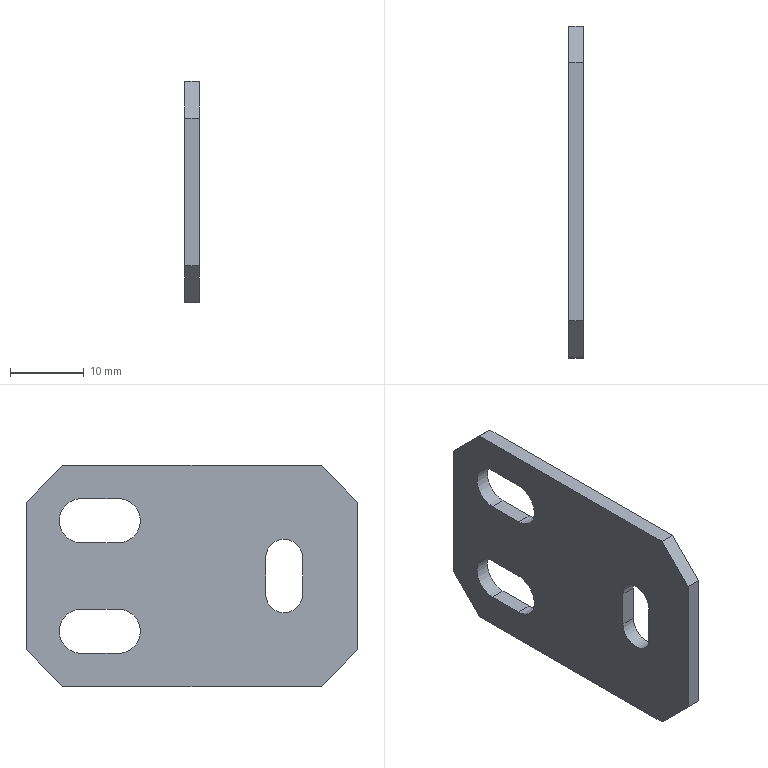Part | NX | features 5003_214_Bracket 2 | 1 solid | 22 faces | box 2 x 45 x 30 mm | volume 2278 mm3 | plane 16 | cylinder 6 | commonest cylinder face diameters 6 x4 5 x2
STEP:
#1=CARTESIAN_POINT('',(-198.775,-594.1,-44.5));
#2=VERTEX_POINT('',#1);
#3=CARTESIAN_POINT('',(-198.775,-594.1,-39.5));
#4=VERTEX_POINT('',#3);
#5=CARTESIAN_POINT('',(-198.775,-594.1,-44.5));
#6=DIRECTION('',(0.,0.,1.));
#7=VECTOR('',#6,1000.);
#8=LINE('',#5,#7);
#9=EDGE_CURVE('',#2,#4,#8,.T.);
#10=ORIENTED_EDGE('',*,*,#9,.F.);
#11=CARTESIAN_POINT('',(-198.775,-589.1,-44.5));
#12=VERTEX_POINT('',#11);
#13=CARTESIAN_POINT('',(-198.775,-591.6,-44.5));
#14=DIRECTION('',(-1.,0.,0.));
#15=DIRECTION('',(0.,0.,1.));
#16=AXIS2_PLACEMENT_3D('',#13,#14,#15);
#17=CIRCLE('',#16,2.5);
#18=EDGE_CURVE('',#12,#2,#17,.T.);
#19=ORIENTED_EDGE('',*,*,#18,.F.);
#20=CARTESIAN_POINT('',(-198.775,-589.1,-39.5));
#21=VERTEX_POINT('',#20);
#22=CARTESIAN_POINT('',(-198.775,-589.1,-44.5));
#23=DIRECTION('',(0.,0.,-1.));
#24=VECTOR('',#23,1000.);
#25=LINE('',#22,#24);
#26=EDGE_CURVE('',#21,#12,#25,.T.);
#27=ORIENTED_EDGE('',*,*,#26,.F.);
#28=CARTESIAN_POINT('',(-198.775,-591.6,-39.5));
#29=DIRECTION('',(-1.,0.,0.));
#30=DIRECTION('',(0.,0.,1.));
#31=AXIS2_PLACEMENT_3D('',#28,#29,#30);
#32=CIRCLE('',#31,2.5);
#33=EDGE_CURVE('',#4,#21,#32,.T.);
#34=ORIENTED_EDGE('',*,*,#33,.F.);
#35=EDGE_LOOP('',(#10,#19,#27,#34));
#36=FACE_BOUND('',#35,.T.);
#37=CARTESIAN_POINT('',(-198.775,-569.1,-52.5));
#38=VERTEX_POINT('',#37);
#39=CARTESIAN_POINT('',(-198.775,-569.1,-46.5));
#40=VERTEX_POINT('',#39);
#41=CARTESIAN_POINT('',(-198.775,-569.1,-49.5));
#42=DIRECTION('',(-1.,0.,0.));
#43=DIRECTION('',(0.,0.,1.));
#44=AXIS2_PLACEMENT_3D('',#41,#42,#43);
#45=CIRCLE('',#44,3.);
#46=EDGE_CURVE('',#38,#40,#45,.T.);
#47=ORIENTED_EDGE('',*,*,#46,.F.);
#48=CARTESIAN_POINT('',(-198.775,-564.1,-52.5));
#49=VERTEX_POINT('',#48);
#50=CARTESIAN_POINT('',(-198.775,-569.1,-52.5));
#51=DIRECTION('',(0.,-1.,0.));
#52=VECTOR('',#51,1000.);
#53=LINE('',#50,#52);
#54=EDGE_CURVE('',#49,#38,#53,.T.);
#55=ORIENTED_EDGE('',*,*,#54,.F.);
#56=CARTESIAN_POINT('',(-198.775,-564.1,-46.5));
#57=VERTEX_POINT('',#56);
#58=CARTESIAN_POINT('',(-198.775,-564.1,-49.5));
#59=DIRECTION('',(-1.,0.,0.));
#60=DIRECTION('',(0.,0.,1.));
#61=AXIS2_PLACEMENT_3D('',#58,#59,#60);
#62=CIRCLE('',#61,3.);
#63=EDGE_CURVE('',#57,#49,#62,.T.);
#64=ORIENTED_EDGE('',*,*,#63,.F.);
#65=CARTESIAN_POINT('',(-198.775,-564.1,-46.5));
#66=DIRECTION('',(0.,1.,0.));
#67=VECTOR('',#66,1000.);
#68=LINE('',#65,#67);
#69=EDGE_CURVE('',#40,#57,#68,.T.);
#70=ORIENTED_EDGE('',*,*,#69,.F.);
#71=EDGE_LOOP('',(#47,#55,#64,#70));
#72=FACE_BOUND('',#71,.T.);
#73=CARTESIAN_POINT('',(-198.775,-601.6,-52.));
#74=VERTEX_POINT('',#73);
#75=CARTESIAN_POINT('',(-198.775,-601.6,-32.));
#76=VERTEX_POINT('',#75);
#77=CARTESIAN_POINT('',(-198.775,-601.6,-27.));
#78=DIRECTION('',(0.,0.,1.));
#79=VECTOR('',#78,1000.);
#80=LINE('',#77,#79);
#81=EDGE_CURVE('',#74,#76,#80,.T.);
#82=ORIENTED_EDGE('',*,*,#81,.T.);
#83=CARTESIAN_POINT('',(-198.775,-596.6,-27.));
#84=VERTEX_POINT('',#83);
#85=CARTESIAN_POINT('',(-198.775,-596.6,-27.));
#86=DIRECTION('',(0.,-0.7071,-0.7071));
#87=VECTOR('',#86,1000.);
#88=LINE('',#85,#87);
#89=EDGE_CURVE('',#76,#84,#88,.F.);
#90=ORIENTED_EDGE('',*,*,#89,.T.);
#91=CARTESIAN_POINT('',(-198.775,-561.6,-27.));
#92=VERTEX_POINT('',#91);
#93=CARTESIAN_POINT('',(-198.775,-601.6,-27.));
#94=DIRECTION('',(0.,1.,0.));
#95=VECTOR('',#94,1000.);
#96=LINE('',#93,#95);
#97=EDGE_CURVE('',#84,#92,#96,.T.);
#98=ORIENTED_EDGE('',*,*,#97,.T.);
#99=CARTESIAN_POINT('',(-198.775,-556.6,-32.));
#100=VERTEX_POINT('',#99);
#101=CARTESIAN_POINT('',(-198.775,-556.6,-32.));
#102=DIRECTION('',(0.,-0.7071,0.7071));
#103=VECTOR('',#102,1000.);
#104=LINE('',#101,#103);
#105=EDGE_CURVE('',#92,#100,#104,.F.);
#106=ORIENTED_EDGE('',*,*,#105,.T.);
#107=CARTESIAN_POINT('',(-198.775,-556.6,-52.));
#108=VERTEX_POINT('',#107);
#109=CARTESIAN_POINT('',(-198.775,-556.6,-27.));
#110=DIRECTION('',(0.,0.,-1.));
#111=VECTOR('',#110,1000.);
#112=LINE('',#109,#111);
#113=EDGE_CURVE('',#100,#108,#112,.T.);
#114=ORIENTED_EDGE('',*,*,#113,.T.);
#115=CARTESIAN_POINT('',(-198.775,-561.6,-57.));
#116=VERTEX_POINT('',#115);
#117=CARTESIAN_POINT('',(-198.775,-561.6,-57.));
#118=DIRECTION('',(0.,0.7071,0.7071));
#119=VECTOR('',#118,1000.);
#120=LINE('',#117,#119);
#121=EDGE_CURVE('',#108,#116,#120,.F.);
#122=ORIENTED_EDGE('',*,*,#121,.T.);
#123=CARTESIAN_POINT('',(-198.775,-596.6,-57.));
#124=VERTEX_POINT('',#123);
#125=CARTESIAN_POINT('',(-198.775,-601.6,-57.));
#126=DIRECTION('',(0.,-1.,0.));
#127=VECTOR('',#126,1000.);
#128=LINE('',#125,#127);
#129=EDGE_CURVE('',#116,#124,#128,.T.);
#130=ORIENTED_EDGE('',*,*,#129,.T.);
#131=CARTESIAN_POINT('',(-198.775,-601.6,-52.));
#132=DIRECTION('',(0.,0.7071,-0.7071));
#133=VECTOR('',#132,1000.);
#134=LINE('',#131,#133);
#135=EDGE_CURVE('',#124,#74,#134,.F.);
#136=ORIENTED_EDGE('',*,*,#135,.T.);
#137=EDGE_LOOP('',(#82,#90,#98,#106,#114,#122,#130,#136));
#138=FACE_BOUND('',#137,.T.);
#139=CARTESIAN_POINT('',(-198.775,-569.1,-37.5));
#140=VERTEX_POINT('',#139);
#141=CARTESIAN_POINT('',(-198.775,-569.1,-31.5));
#142=VERTEX_POINT('',#141);
#143=CARTESIAN_POINT('',(-198.775,-569.1,-34.5));
#144=DIRECTION('',(-1.,0.,0.));
#145=DIRECTION('',(0.,0.,1.));
#146=AXIS2_PLACEMENT_3D('',#143,#144,#145);
#147=CIRCLE('',#146,3.);
#148=EDGE_CURVE('',#140,#142,#147,.T.);
#149=ORIENTED_EDGE('',*,*,#148,.F.);
#150=CARTESIAN_POINT('',(-198.775,-564.1,-37.5));
#151=VERTEX_POINT('',#150);
#152=CARTESIAN_POINT('',(-198.775,-569.1,-37.5));
#153=DIRECTION('',(0.,-1.,0.));
#154=VECTOR('',#153,1000.);
#155=LINE('',#152,#154);
#156=EDGE_CURVE('',#151,#140,#155,.T.);
#157=ORIENTED_EDGE('',*,*,#156,.F.);
#158=CARTESIAN_POINT('',(-198.775,-564.1,-31.5));
#159=VERTEX_POINT('',#158);
#160=CARTESIAN_POINT('',(-198.775,-564.1,-34.5));
#161=DIRECTION('',(-1.,0.,0.));
#162=DIRECTION('',(0.,0.,1.));
#163=AXIS2_PLACEMENT_3D('',#160,#161,#162);
#164=CIRCLE('',#163,3.);
#165=EDGE_CURVE('',#159,#151,#164,.T.);
#166=ORIENTED_EDGE('',*,*,#165,.F.);
#167=CARTESIAN_POINT('',(-198.775,-564.1,-31.5));
#168=DIRECTION('',(0.,1.,0.));
#169=VECTOR('',#168,1000.);
#170=LINE('',#167,#169);
#171=EDGE_CURVE('',#142,#159,#170,.T.);
#172=ORIENTED_EDGE('',*,*,#171,.F.);
#173=EDGE_LOOP('',(#149,#157,#166,#172));
#174=FACE_BOUND('',#173,.T.);
#175=CARTESIAN_POINT('',(-198.775,-601.6,-27.));
#176=DIRECTION('',(1.,0.,0.));
#177=DIRECTION('',(0.,0.,-1.));
#178=AXIS2_PLACEMENT_3D('',#175,#176,#177);
#179=PLANE('',#178);
#180=ADVANCED_FACE('',(#36,#72,#138,#174),#179,.F.);
#181=CARTESIAN_POINT('',(-196.775,-589.1,-44.5));
#182=VERTEX_POINT('',#181);
#183=CARTESIAN_POINT('',(-196.775,-594.1,-44.5));
#184=VERTEX_POINT('',#183);
#185=CARTESIAN_POINT('',(-196.775,-591.6,-44.5));
#186=DIRECTION('',(-1.,0.,0.));
#187=DIRECTION('',(0.,0.,1.));
#188=AXIS2_PLACEMENT_3D('',#185,#186,#187);
#189=CIRCLE('',#188,2.5);
#190=EDGE_CURVE('',#182,#184,#189,.T.);
#191=ORIENTED_EDGE('',*,*,#190,.T.);
#192=CARTESIAN_POINT('',(-196.775,-594.1,-39.5));
#193=VERTEX_POINT('',#192);
#194=CARTESIAN_POINT('',(-196.775,-594.1,-44.5));
#195=DIRECTION('',(0.,0.,1.));
#196=VECTOR('',#195,1000.);
#197=LINE('',#194,#196);
#198=EDGE_CURVE('',#184,#193,#197,.T.);
#199=ORIENTED_EDGE('',*,*,#198,.T.);
#200=CARTESIAN_POINT('',(-196.775,-589.1,-39.5));
#201=VERTEX_POINT('',#200);
#202=CARTESIAN_POINT('',(-196.775,-591.6,-39.5));
#203=DIRECTION('',(-1.,0.,0.));
#204=DIRECTION('',(0.,0.,1.));
#205=AXIS2_PLACEMENT_3D('',#202,#203,#204);
#206=CIRCLE('',#205,2.5);
#207=EDGE_CURVE('',#193,#201,#206,.T.);
#208=ORIENTED_EDGE('',*,*,#207,.T.);
#209=CARTESIAN_POINT('',(-196.775,-589.1,-44.5));
#210=DIRECTION('',(0.,0.,-1.));
#211=VECTOR('',#210,1000.);
#212=LINE('',#209,#211);
#213=EDGE_CURVE('',#201,#182,#212,.T.);
#214=ORIENTED_EDGE('',*,*,#213,.T.);
#215=EDGE_LOOP('',(#191,#199,#208,#214));
#216=FACE_BOUND('',#215,.T.);
#217=CARTESIAN_POINT('',(-196.775,-564.1,-52.5));
#218=VERTEX_POINT('',#217);
#219=CARTESIAN_POINT('',(-196.775,-569.1,-52.5));
#220=VERTEX_POINT('',#219);
#221=CARTESIAN_POINT('',(-196.775,-569.1,-52.5));
#222=DIRECTION('',(0.,-1.,0.));
#223=VECTOR('',#222,1000.);
#224=LINE('',#221,#223);
#225=EDGE_CURVE('',#218,#220,#224,.T.);
#226=ORIENTED_EDGE('',*,*,#225,.T.);
#227=CARTESIAN_POINT('',(-196.775,-569.1,-46.5));
#228=VERTEX_POINT('',#227);
#229=CARTESIAN_POINT('',(-196.775,-569.1,-49.5));
#230=DIRECTION('',(-1.,0.,0.));
#231=DIRECTION('',(0.,0.,1.));
#232=AXIS2_PLACEMENT_3D('',#229,#230,#231);
#233=CIRCLE('',#232,3.);
#234=EDGE_CURVE('',#220,#228,#233,.T.);
#235=ORIENTED_EDGE('',*,*,#234,.T.);
#236=CARTESIAN_POINT('',(-196.775,-564.1,-46.5));
#237=VERTEX_POINT('',#236);
#238=CARTESIAN_POINT('',(-196.775,-564.1,-46.5));
#239=DIRECTION('',(0.,1.,0.));
#240=VECTOR('',#239,1000.);
#241=LINE('',#238,#240);
#242=EDGE_CURVE('',#228,#237,#241,.T.);
#243=ORIENTED_EDGE('',*,*,#242,.T.);
#244=CARTESIAN_POINT('',(-196.775,-564.1,-49.5));
#245=DIRECTION('',(-1.,0.,0.));
#246=DIRECTION('',(0.,0.,1.));
#247=AXIS2_PLACEMENT_3D('',#244,#245,#246);
#248=CIRCLE('',#247,3.);
#249=EDGE_CURVE('',#237,#218,#248,.T.);
#250=ORIENTED_EDGE('',*,*,#249,.T.);
#251=EDGE_LOOP('',(#226,#235,#243,#250));
#252=FACE_BOUND('',#251,.T.);
#253=CARTESIAN_POINT('',(-196.775,-596.6,-27.));
#254=VERTEX_POINT('',#253);
#255=CARTESIAN_POINT('',(-196.775,-561.6,-27.));
#256=VERTEX_POINT('',#255);
#257=CARTESIAN_POINT('',(-196.775,-601.6,-27.));
#258=DIRECTION('',(0.,1.,0.));
#259=VECTOR('',#258,1000.);
#260=LINE('',#257,#259);
#261=EDGE_CURVE('',#254,#256,#260,.T.);
#262=ORIENTED_EDGE('',*,*,#261,.F.);
#263=CARTESIAN_POINT('',(-196.775,-601.6,-32.));
#264=VERTEX_POINT('',#263);
#265=CARTESIAN_POINT('',(-196.775,-599.1,-29.5));
#266=DIRECTION('',(0.,0.7071,0.7071));
#267=VECTOR('',#266,1000.);
#268=LINE('',#265,#267);
#269=EDGE_CURVE('',#254,#264,#268,.F.);
#270=ORIENTED_EDGE('',*,*,#269,.T.);
#271=CARTESIAN_POINT('',(-196.775,-601.6,-52.));
#272=VERTEX_POINT('',#271);
#273=CARTESIAN_POINT('',(-196.775,-601.6,-27.));
#274=DIRECTION('',(0.,0.,1.));
#275=VECTOR('',#274,1000.);
#276=LINE('',#273,#275);
#277=EDGE_CURVE('',#272,#264,#276,.T.);
#278=ORIENTED_EDGE('',*,*,#277,.F.);
#279=CARTESIAN_POINT('',(-196.775,-596.6,-57.));
#280=VERTEX_POINT('',#279);
#281=CARTESIAN_POINT('',(-196.775,-614.1,-39.5));
#282=DIRECTION('',(0.,-0.7071,0.7071));
#283=VECTOR('',#282,1000.);
#284=LINE('',#281,#283);
#285=EDGE_CURVE('',#272,#280,#284,.F.);
#286=ORIENTED_EDGE('',*,*,#285,.T.);
#287=CARTESIAN_POINT('',(-196.775,-561.6,-57.));
#288=VERTEX_POINT('',#287);
#289=CARTESIAN_POINT('',(-196.775,-601.6,-57.));
#290=DIRECTION('',(0.,-1.,0.));
#291=VECTOR('',#290,1000.);
#292=LINE('',#289,#291);
#293=EDGE_CURVE('',#288,#280,#292,.T.);
#294=ORIENTED_EDGE('',*,*,#293,.F.);
#295=CARTESIAN_POINT('',(-196.775,-556.6,-52.));
#296=VERTEX_POINT('',#295);
#297=CARTESIAN_POINT('',(-196.775,-566.6,-62.));
#298=DIRECTION('',(0.,-0.7071,-0.7071));
#299=VECTOR('',#298,1000.);
#300=LINE('',#297,#299);
#301=EDGE_CURVE('',#288,#296,#300,.F.);
#302=ORIENTED_EDGE('',*,*,#301,.T.);
#303=CARTESIAN_POINT('',(-196.775,-556.6,-32.));
#304=VERTEX_POINT('',#303);
#305=CARTESIAN_POINT('',(-196.775,-556.6,-27.));
#306=DIRECTION('',(0.,0.,-1.));
#307=VECTOR('',#306,1000.);
#308=LINE('',#305,#307);
#309=EDGE_CURVE('',#304,#296,#308,.T.);
#310=ORIENTED_EDGE('',*,*,#309,.F.);
#311=CARTESIAN_POINT('',(-196.775,-581.6,-7.));
#312=DIRECTION('',(0.,0.7071,-0.7071));
#313=VECTOR('',#312,1000.);
#314=LINE('',#311,#313);
#315=EDGE_CURVE('',#304,#256,#314,.F.);
#316=ORIENTED_EDGE('',*,*,#315,.T.);
#317=EDGE_LOOP('',(#262,#270,#278,#286,#294,#302,#310,#316));
#318=FACE_BOUND('',#317,.T.);
#319=CARTESIAN_POINT('',(-196.775,-564.1,-37.5));
#320=VERTEX_POINT('',#319);
#321=CARTESIAN_POINT('',(-196.775,-569.1,-37.5));
#322=VERTEX_POINT('',#321);
#323=CARTESIAN_POINT('',(-196.775,-569.1,-37.5));
#324=DIRECTION('',(0.,-1.,0.));
#325=VECTOR('',#324,1000.);
#326=LINE('',#323,#325);
#327=EDGE_CURVE('',#320,#322,#326,.T.);
#328=ORIENTED_EDGE('',*,*,#327,.T.);
#329=CARTESIAN_POINT('',(-196.775,-569.1,-31.5));
#330=VERTEX_POINT('',#329);
#331=CARTESIAN_POINT('',(-196.775,-569.1,-34.5));
#332=DIRECTION('',(-1.,0.,0.));
#333=DIRECTION('',(0.,0.,1.));
#334=AXIS2_PLACEMENT_3D('',#331,#332,#333);
#335=CIRCLE('',#334,3.);
#336=EDGE_CURVE('',#322,#330,#335,.T.);
#337=ORIENTED_EDGE('',*,*,#336,.T.);
#338=CARTESIAN_POINT('',(-196.775,-564.1,-31.5));
#339=VERTEX_POINT('',#338);
#340=CARTESIAN_POINT('',(-196.775,-564.1,-31.5));
#341=DIRECTION('',(0.,1.,0.));
#342=VECTOR('',#341,1000.);
#343=LINE('',#340,#342);
#344=EDGE_CURVE('',#330,#339,#343,.T.);
#345=ORIENTED_EDGE('',*,*,#344,.T.);
#346=CARTESIAN_POINT('',(-196.775,-564.1,-34.5));
#347=DIRECTION('',(-1.,0.,0.));
#348=DIRECTION('',(0.,0.,1.));
#349=AXIS2_PLACEMENT_3D('',#346,#347,#348);
#350=CIRCLE('',#349,3.);
#351=EDGE_CURVE('',#339,#320,#350,.T.);
#352=ORIENTED_EDGE('',*,*,#351,.T.);
#353=EDGE_LOOP('',(#328,#337,#345,#352));
#354=FACE_BOUND('',#353,.T.);
#355=CARTESIAN_POINT('',(-196.775,-601.6,-27.));
#356=DIRECTION('',(1.,0.,0.));
#357=DIRECTION('',(0.,0.,-1.));
#358=AXIS2_PLACEMENT_3D('',#355,#356,#357);
#359=PLANE('',#358);
#360=ADVANCED_FACE('',(#216,#252,#318,#354),#359,.T.);
#361=ORIENTED_EDGE('',*,*,#277,.T.);
#362=CARTESIAN_POINT('',(-198.775,-601.6,-32.));
#363=DIRECTION('',(-1.,0.,0.));
#364=VECTOR('',#363,1000.);
#365=LINE('',#362,#364);
#366=EDGE_CURVE('',#264,#76,#365,.T.);
#367=ORIENTED_EDGE('',*,*,#366,.T.);
#368=ORIENTED_EDGE('',*,*,#81,.F.);
#369=CARTESIAN_POINT('',(-198.775,-601.6,-52.));
#370=DIRECTION('',(1.,0.,0.));
#371=VECTOR('',#370,1000.);
#372=LINE('',#369,#371);
#373=EDGE_CURVE('',#74,#272,#372,.T.);
#374=ORIENTED_EDGE('',*,*,#373,.T.);
#375=EDGE_LOOP('',(#361,#367,#368,#374));
#376=FACE_BOUND('',#375,.T.);
#377=CARTESIAN_POINT('',(-198.775,-601.6,-27.));
#378=DIRECTION('',(0.,1.,0.));
#379=DIRECTION('',(0.,0.,-1.));
#380=AXIS2_PLACEMENT_3D('',#377,#378,#379);
#381=PLANE('',#380);
#382=ADVANCED_FACE('',(#376),#381,.F.);
#383=ORIENTED_EDGE('',*,*,#97,.F.);
#384=CARTESIAN_POINT('',(-198.775,-596.6,-27.));
#385=DIRECTION('',(1.,0.,0.));
#386=VECTOR('',#385,1000.);
#387=LINE('',#384,#386);
#388=EDGE_CURVE('',#84,#254,#387,.T.);
#389=ORIENTED_EDGE('',*,*,#388,.T.);
#390=ORIENTED_EDGE('',*,*,#261,.T.);
#391=CARTESIAN_POINT('',(-198.775,-561.6,-27.));
#392=DIRECTION('',(-1.,0.,0.));
#393=VECTOR('',#392,1000.);
#394=LINE('',#391,#393);
#395=EDGE_CURVE('',#256,#92,#394,.T.);
#396=ORIENTED_EDGE('',*,*,#395,.T.);
#397=EDGE_LOOP('',(#383,#389,#390,#396));
#398=FACE_BOUND('',#397,.T.);
#399=CARTESIAN_POINT('',(-198.775,-601.6,-27.));
#400=DIRECTION('',(0.,0.,-1.));
#401=DIRECTION('',(0.,-1.,0.));
#402=AXIS2_PLACEMENT_3D('',#399,#400,#401);
#403=PLANE('',#402);
#404=ADVANCED_FACE('',(#398),#403,.F.);
#405=ORIENTED_EDGE('',*,*,#113,.F.);
#406=CARTESIAN_POINT('',(-198.775,-556.6,-32.));
#407=DIRECTION('',(1.,0.,0.));
#408=VECTOR('',#407,1000.);
#409=LINE('',#406,#408);
#410=EDGE_CURVE('',#100,#304,#409,.T.);
#411=ORIENTED_EDGE('',*,*,#410,.T.);
#412=ORIENTED_EDGE('',*,*,#309,.T.);
#413=CARTESIAN_POINT('',(-198.775,-556.6,-52.));
#414=DIRECTION('',(-1.,0.,0.));
#415=VECTOR('',#414,1000.);
#416=LINE('',#413,#415);
#417=EDGE_CURVE('',#296,#108,#416,.T.);
#418=ORIENTED_EDGE('',*,*,#417,.T.);
#419=EDGE_LOOP('',(#405,#411,#412,#418));
#420=FACE_BOUND('',#419,.T.);
#421=CARTESIAN_POINT('',(-198.775,-556.6,-27.));
#422=DIRECTION('',(0.,-1.,0.));
#423=DIRECTION('',(0.,0.,1.));
#424=AXIS2_PLACEMENT_3D('',#421,#422,#423);
#425=PLANE('',#424);
#426=ADVANCED_FACE('',(#420),#425,.F.);
#427=ORIENTED_EDGE('',*,*,#129,.F.);
#428=CARTESIAN_POINT('',(-198.775,-561.6,-57.));
#429=DIRECTION('',(1.,0.,0.));
#430=VECTOR('',#429,1000.);
#431=LINE('',#428,#430);
#432=EDGE_CURVE('',#116,#288,#431,.T.);
#433=ORIENTED_EDGE('',*,*,#432,.T.);
#434=ORIENTED_EDGE('',*,*,#293,.T.);
#435=CARTESIAN_POINT('',(-198.775,-596.6,-57.));
#436=DIRECTION('',(-1.,0.,0.));
#437=VECTOR('',#436,1000.);
#438=LINE('',#435,#437);
#439=EDGE_CURVE('',#280,#124,#438,.T.);
#440=ORIENTED_EDGE('',*,*,#439,.T.);
#441=EDGE_LOOP('',(#427,#433,#434,#440));
#442=FACE_BOUND('',#441,.T.);
#443=CARTESIAN_POINT('',(-198.775,-601.6,-57.));
#444=DIRECTION('',(0.,0.,1.));
#445=DIRECTION('',(0.,1.,0.));
#446=AXIS2_PLACEMENT_3D('',#443,#444,#445);
#447=PLANE('',#446);
#448=ADVANCED_FACE('',(#442),#447,.F.);
#449=ORIENTED_EDGE('',*,*,#234,.F.);
#450=CARTESIAN_POINT('',(-198.775,-569.1,-52.5));
#451=DIRECTION('',(1.,0.,0.));
#452=VECTOR('',#451,1000.);
#453=LINE('',#450,#452);
#454=EDGE_CURVE('',#38,#220,#453,.T.);
#455=ORIENTED_EDGE('',*,*,#454,.F.);
#456=ORIENTED_EDGE('',*,*,#46,.T.);
#457=CARTESIAN_POINT('',(-198.775,-569.1,-46.5));
#458=DIRECTION('',(1.,0.,0.));
#459=VECTOR('',#458,1000.);
#460=LINE('',#457,#459);
#461=EDGE_CURVE('',#40,#228,#460,.T.);
#462=ORIENTED_EDGE('',*,*,#461,.T.);
#463=EDGE_LOOP('',(#449,#455,#456,#462));
#464=FACE_BOUND('',#463,.T.);
#465=CARTESIAN_POINT('',(-198.775,-569.1,-49.5));
#466=DIRECTION('',(1.,0.,0.));
#467=DIRECTION('',(0.,0.,-1.));
#468=AXIS2_PLACEMENT_3D('',#465,#466,#467);
#469=CYLINDRICAL_SURFACE('',#468,3.);
#470=ADVANCED_FACE('',(#464),#469,.F.);
#471=ORIENTED_EDGE('',*,*,#242,.F.);
#472=ORIENTED_EDGE('',*,*,#461,.F.);
#473=ORIENTED_EDGE('',*,*,#69,.T.);
#474=CARTESIAN_POINT('',(-198.775,-564.1,-46.5));
#475=DIRECTION('',(1.,0.,0.));
#476=VECTOR('',#475,1000.);
#477=LINE('',#474,#476);
#478=EDGE_CURVE('',#57,#237,#477,.T.);
#479=ORIENTED_EDGE('',*,*,#478,.T.);
#480=EDGE_LOOP('',(#471,#472,#473,#479));
#481=FACE_BOUND('',#480,.T.);
#482=CARTESIAN_POINT('',(-198.775,-564.1,-46.5));
#483=DIRECTION('',(0.,0.,-1.));
#484=DIRECTION('',(0.,-1.,0.));
#485=AXIS2_PLACEMENT_3D('',#482,#483,#484);
#486=PLANE('',#485);
#487=ADVANCED_FACE('',(#481),#486,.T.);
#488=ORIENTED_EDGE('',*,*,#249,.F.);
#489=ORIENTED_EDGE('',*,*,#478,.F.);
#490=ORIENTED_EDGE('',*,*,#63,.T.);
#491=CARTESIAN_POINT('',(-198.775,-564.1,-52.5));
#492=DIRECTION('',(1.,0.,0.));
#493=VECTOR('',#492,1000.);
#494=LINE('',#491,#493);
#495=EDGE_CURVE('',#49,#218,#494,.T.);
#496=ORIENTED_EDGE('',*,*,#495,.T.);
#497=EDGE_LOOP('',(#488,#489,#490,#496));
#498=FACE_BOUND('',#497,.T.);
#499=CARTESIAN_POINT('',(-198.775,-564.1,-49.5));
#500=DIRECTION('',(1.,0.,0.));
#501=DIRECTION('',(0.,0.,-1.));
#502=AXIS2_PLACEMENT_3D('',#499,#500,#501);
#503=CYLINDRICAL_SURFACE('',#502,3.);
#504=ADVANCED_FACE('',(#498),#503,.F.);
#505=ORIENTED_EDGE('',*,*,#225,.F.);
#506=ORIENTED_EDGE('',*,*,#495,.F.);
#507=ORIENTED_EDGE('',*,*,#54,.T.);
#508=ORIENTED_EDGE('',*,*,#454,.T.);
#509=EDGE_LOOP('',(#505,#506,#507,#508));
#510=FACE_BOUND('',#509,.T.);
#511=CARTESIAN_POINT('',(-198.775,-569.1,-52.5));
#512=DIRECTION('',(0.,0.,1.));
#513=DIRECTION('',(0.,1.,0.));
#514=AXIS2_PLACEMENT_3D('',#511,#512,#513);
#515=PLANE('',#514);
#516=ADVANCED_FACE('',(#510),#515,.T.);
#517=ORIENTED_EDGE('',*,*,#336,.F.);
#518=CARTESIAN_POINT('',(-198.775,-569.1,-37.5));
#519=DIRECTION('',(1.,0.,0.));
#520=VECTOR('',#519,1000.);
#521=LINE('',#518,#520);
#522=EDGE_CURVE('',#140,#322,#521,.T.);
#523=ORIENTED_EDGE('',*,*,#522,.F.);
#524=ORIENTED_EDGE('',*,*,#148,.T.);
#525=CARTESIAN_POINT('',(-198.775,-569.1,-31.5));
#526=DIRECTION('',(1.,0.,0.));
#527=VECTOR('',#526,1000.);
#528=LINE('',#525,#527);
#529=EDGE_CURVE('',#142,#330,#528,.T.);
#530=ORIENTED_EDGE('',*,*,#529,.T.);
#531=EDGE_LOOP('',(#517,#523,#524,#530));
#532=FACE_BOUND('',#531,.T.);
#533=CARTESIAN_POINT('',(-198.775,-569.1,-34.5));
#534=DIRECTION('',(1.,0.,0.));
#535=DIRECTION('',(0.,0.,-1.));
#536=AXIS2_PLACEMENT_3D('',#533,#534,#535);
#537=CYLINDRICAL_SURFACE('',#536,3.);
#538=ADVANCED_FACE('',(#532),#537,.F.);
#539=ORIENTED_EDGE('',*,*,#344,.F.);
#540=ORIENTED_EDGE('',*,*,#529,.F.);
#541=ORIENTED_EDGE('',*,*,#171,.T.);
#542=CARTESIAN_POINT('',(-198.775,-564.1,-31.5));
#543=DIRECTION('',(1.,0.,0.));
#544=VECTOR('',#543,1000.);
#545=LINE('',#542,#544);
#546=EDGE_CURVE('',#159,#339,#545,.T.);
#547=ORIENTED_EDGE('',*,*,#546,.T.);
#548=EDGE_LOOP('',(#539,#540,#541,#547));
#549=FACE_BOUND('',#548,.T.);
#550=CARTESIAN_POINT('',(-198.775,-564.1,-31.5));
#551=DIRECTION('',(0.,0.,-1.));
#552=DIRECTION('',(0.,-1.,0.));
#553=AXIS2_PLACEMENT_3D('',#550,#551,#552);
#554=PLANE('',#553);
#555=ADVANCED_FACE('',(#549),#554,.T.);
#556=ORIENTED_EDGE('',*,*,#351,.F.);
#557=ORIENTED_EDGE('',*,*,#546,.F.);
#558=ORIENTED_EDGE('',*,*,#165,.T.);
#559=CARTESIAN_POINT('',(-198.775,-564.1,-37.5));
#560=DIRECTION('',(1.,0.,0.));
#561=VECTOR('',#560,1000.);
#562=LINE('',#559,#561);
#563=EDGE_CURVE('',#151,#320,#562,.T.);
#564=ORIENTED_EDGE('',*,*,#563,.T.);
#565=EDGE_LOOP('',(#556,#557,#558,#564));
#566=FACE_BOUND('',#565,.T.);
#567=CARTESIAN_POINT('',(-198.775,-564.1,-34.5));
#568=DIRECTION('',(1.,0.,0.));
#569=DIRECTION('',(0.,0.,-1.));
#570=AXIS2_PLACEMENT_3D('',#567,#568,#569);
#571=CYLINDRICAL_SURFACE('',#570,3.);
#572=ADVANCED_FACE('',(#566),#571,.F.);
#573=ORIENTED_EDGE('',*,*,#327,.F.);
#574=ORIENTED_EDGE('',*,*,#563,.F.);
#575=ORIENTED_EDGE('',*,*,#156,.T.);
#576=ORIENTED_EDGE('',*,*,#522,.T.);
#577=EDGE_LOOP('',(#573,#574,#575,#576));
#578=FACE_BOUND('',#577,.T.);
#579=CARTESIAN_POINT('',(-198.775,-569.1,-37.5));
#580=DIRECTION('',(0.,0.,1.));
#581=DIRECTION('',(0.,1.,0.));
#582=AXIS2_PLACEMENT_3D('',#579,#580,#581);
#583=PLANE('',#582);
#584=ADVANCED_FACE('',(#578),#583,.T.);
#585=ORIENTED_EDGE('',*,*,#18,.T.);
#586=CARTESIAN_POINT('',(-196.775,-594.1,-44.5));
#587=DIRECTION('',(-1.,0.,0.));
#588=VECTOR('',#587,1000.);
#589=LINE('',#586,#588);
#590=EDGE_CURVE('',#184,#2,#589,.T.);
#591=ORIENTED_EDGE('',*,*,#590,.F.);
#592=ORIENTED_EDGE('',*,*,#190,.F.);
#593=CARTESIAN_POINT('',(-196.775,-589.1,-44.5));
#594=DIRECTION('',(-1.,0.,0.));
#595=VECTOR('',#594,1000.);
#596=LINE('',#593,#595);
#597=EDGE_CURVE('',#182,#12,#596,.T.);
#598=ORIENTED_EDGE('',*,*,#597,.T.);
#599=EDGE_LOOP('',(#585,#591,#592,#598));
#600=FACE_BOUND('',#599,.T.);
#601=CARTESIAN_POINT('',(-196.775,-591.6,-44.5));
#602=DIRECTION('',(-1.,0.,0.));
#603=DIRECTION('',(0.,0.,1.));
#604=AXIS2_PLACEMENT_3D('',#601,#602,#603);
#605=CYLINDRICAL_SURFACE('',#604,2.5);
#606=ADVANCED_FACE('',(#600),#605,.F.);
#607=ORIENTED_EDGE('',*,*,#26,.T.);
#608=ORIENTED_EDGE('',*,*,#597,.F.);
#609=ORIENTED_EDGE('',*,*,#213,.F.);
#610=CARTESIAN_POINT('',(-196.775,-589.1,-39.5));
#611=DIRECTION('',(-1.,0.,0.));
#612=VECTOR('',#611,1000.);
#613=LINE('',#610,#612);
#614=EDGE_CURVE('',#201,#21,#613,.T.);
#615=ORIENTED_EDGE('',*,*,#614,.T.);
#616=EDGE_LOOP('',(#607,#608,#609,#615));
#617=FACE_BOUND('',#616,.T.);
#618=CARTESIAN_POINT('',(-196.775,-589.1,-44.5));
#619=DIRECTION('',(0.,1.,0.));
#620=DIRECTION('',(0.,0.,-1.));
#621=AXIS2_PLACEMENT_3D('',#618,#619,#620);
#622=PLANE('',#621);
#623=ADVANCED_FACE('',(#617),#622,.F.);
#624=ORIENTED_EDGE('',*,*,#33,.T.);
#625=ORIENTED_EDGE('',*,*,#614,.F.);
#626=ORIENTED_EDGE('',*,*,#207,.F.);
#627=CARTESIAN_POINT('',(-196.775,-594.1,-39.5));
#628=DIRECTION('',(-1.,0.,0.));
#629=VECTOR('',#628,1000.);
#630=LINE('',#627,#629);
#631=EDGE_CURVE('',#193,#4,#630,.T.);
#632=ORIENTED_EDGE('',*,*,#631,.T.);
#633=EDGE_LOOP('',(#624,#625,#626,#632));
#634=FACE_BOUND('',#633,.T.);
#635=CARTESIAN_POINT('',(-196.775,-591.6,-39.5));
#636=DIRECTION('',(-1.,0.,0.));
#637=DIRECTION('',(0.,0.,1.));
#638=AXIS2_PLACEMENT_3D('',#635,#636,#637);
#639=CYLINDRICAL_SURFACE('',#638,2.5);
#640=ADVANCED_FACE('',(#634),#639,.F.);
#641=ORIENTED_EDGE('',*,*,#9,.T.);
#642=ORIENTED_EDGE('',*,*,#631,.F.);
#643=ORIENTED_EDGE('',*,*,#198,.F.);
#644=ORIENTED_EDGE('',*,*,#590,.T.);
#645=EDGE_LOOP('',(#641,#642,#643,#644));
#646=FACE_BOUND('',#645,.T.);
#647=CARTESIAN_POINT('',(-196.775,-594.1,-44.5));
#648=DIRECTION('',(0.,-1.,0.));
#649=DIRECTION('',(0.,0.,1.));
#650=AXIS2_PLACEMENT_3D('',#647,#648,#649);
#651=PLANE('',#650);
#652=ADVANCED_FACE('',(#646),#651,.F.);
#653=ORIENTED_EDGE('',*,*,#135,.F.);
#654=ORIENTED_EDGE('',*,*,#439,.F.);
#655=ORIENTED_EDGE('',*,*,#285,.F.);
#656=ORIENTED_EDGE('',*,*,#373,.F.);
#657=EDGE_LOOP('',(#653,#654,#655,#656));
#658=FACE_BOUND('',#657,.T.);
#659=CARTESIAN_POINT('',(-198.775,-601.6,-52.));
#660=DIRECTION('',(0.,0.7071,0.7071));
#661=DIRECTION('',(1.,0.,0.));
#662=AXIS2_PLACEMENT_3D('',#659,#660,#661);
#663=PLANE('',#662);
#664=ADVANCED_FACE('',(#658),#663,.F.);
#665=ORIENTED_EDGE('',*,*,#121,.F.);
#666=ORIENTED_EDGE('',*,*,#417,.F.);
#667=ORIENTED_EDGE('',*,*,#301,.F.);
#668=ORIENTED_EDGE('',*,*,#432,.F.);
#669=EDGE_LOOP('',(#665,#666,#667,#668));
#670=FACE_BOUND('',#669,.T.);
#671=CARTESIAN_POINT('',(-198.775,-561.6,-57.));
#672=DIRECTION('',(0.,-0.7071,0.7071));
#673=DIRECTION('',(1.,0.,0.));
#674=AXIS2_PLACEMENT_3D('',#671,#672,#673);
#675=PLANE('',#674);
#676=ADVANCED_FACE('',(#670),#675,.F.);
#677=ORIENTED_EDGE('',*,*,#105,.F.);
#678=ORIENTED_EDGE('',*,*,#395,.F.);
#679=ORIENTED_EDGE('',*,*,#315,.F.);
#680=ORIENTED_EDGE('',*,*,#410,.F.);
#681=EDGE_LOOP('',(#677,#678,#679,#680));
#682=FACE_BOUND('',#681,.T.);
#683=CARTESIAN_POINT('',(-198.775,-556.6,-32.));
#684=DIRECTION('',(0.,-0.7071,-0.7071));
#685=DIRECTION('',(1.,0.,0.));
#686=AXIS2_PLACEMENT_3D('',#683,#684,#685);
#687=PLANE('',#686);
#688=ADVANCED_FACE('',(#682),#687,.F.);
#689=ORIENTED_EDGE('',*,*,#89,.F.);
#690=ORIENTED_EDGE('',*,*,#366,.F.);
#691=ORIENTED_EDGE('',*,*,#269,.F.);
#692=ORIENTED_EDGE('',*,*,#388,.F.);
#693=EDGE_LOOP('',(#689,#690,#691,#692));
#694=FACE_BOUND('',#693,.T.);
#695=CARTESIAN_POINT('',(-198.775,-596.6,-27.));
#696=DIRECTION('',(0.,0.7071,-0.7071));
#697=DIRECTION('',(1.,0.,0.));
#698=AXIS2_PLACEMENT_3D('',#695,#696,#697);
#699=PLANE('',#698);
#700=ADVANCED_FACE('',(#694),#699,.F.);
#701=CLOSED_SHELL('',(#180,#360,#382,#404,#426,#448,#470,#487,#504,#516,#538,#555,#572,#584,#606,#623,#640,#652,#664,#676,#688,#700));
#702=MANIFOLD_SOLID_BREP('',#701);
#703=(LENGTH_UNIT()NAMED_UNIT(*)SI_UNIT(.MILLI.,.METRE.));
#704=UNCERTAINTY_MEASURE_WITH_UNIT(LENGTH_MEASURE(0.00001),#703,'','');
#705=(NAMED_UNIT(*)PLANE_ANGLE_UNIT()SI_UNIT($,.RADIAN.));
#706=(NAMED_UNIT(*)SI_UNIT($,.STERADIAN.)SOLID_ANGLE_UNIT());
#707=(GEOMETRIC_REPRESENTATION_CONTEXT(3)GLOBAL_UNCERTAINTY_ASSIGNED_CONTEXT((#704))GLOBAL_UNIT_ASSIGNED_CONTEXT((#703,#705,#706))REPRESENTATION_CONTEXT('',''));
#708=ADVANCED_BREP_SHAPE_REPRESENTATION('',(#702),#707);